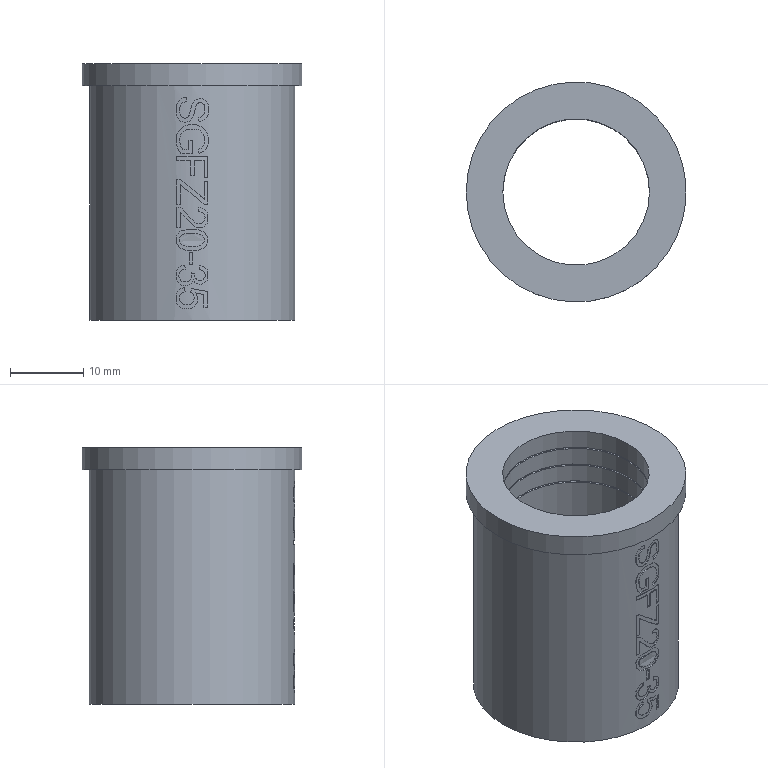Part | NX | features SGFZ20-35_1 2 | 1 solid | 143 faces | box 30 x 30 x 35 mm | volume 10820 mm3 | plane 80 | cylinder 60 | torus 3 | commonest cylinder face diameters 27.8 x9 20 x4 2.533 x2 28 x2 1.198 x1 1.241 x1